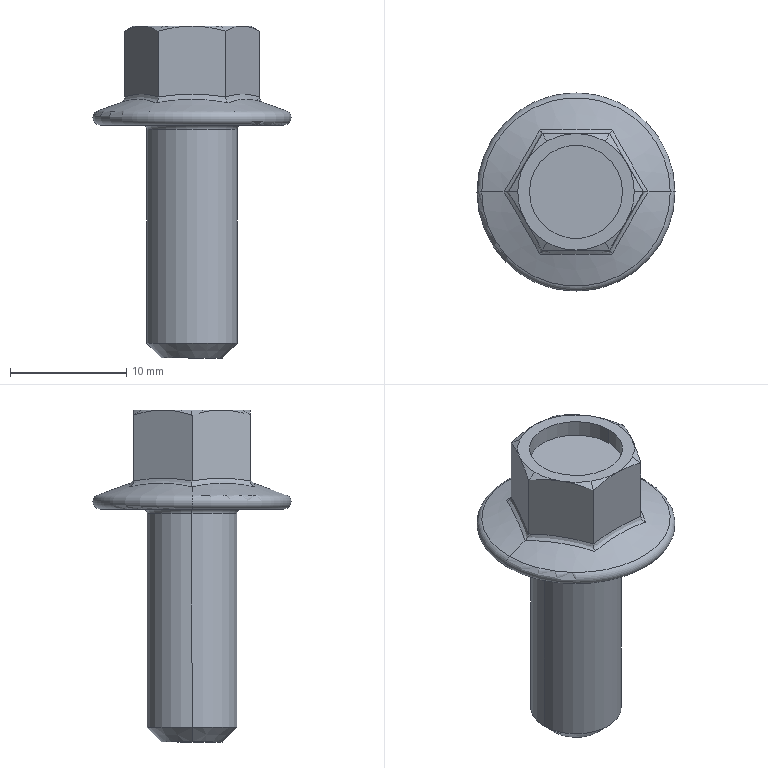Part | SolidWorks | features BaseBody 1 | 1 solid | 40 faces | box 17 x 17 x 28.5 mm | volume 1813 mm3 | cone 16 | plane 10 | spline 6 | cylinder 4 | torus 4 | commonest cylinder face diameters 7.76 x2 8 x2